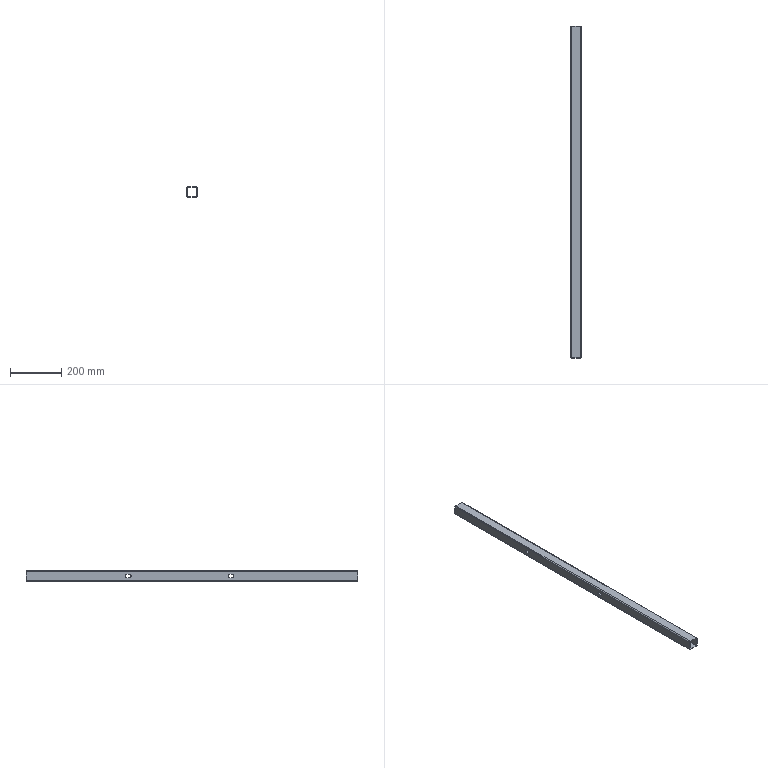Part | STEP file | E3-中转釜护栏7-1立柱主体_Default<As Machined> | 1 solid | 34 faces | box 40 x 1292 x 40 mm | volume 377594 mm3 | plane 18 | cylinder 16 | commonest cylinder face diameters 12 x8 4 x4 8 x4